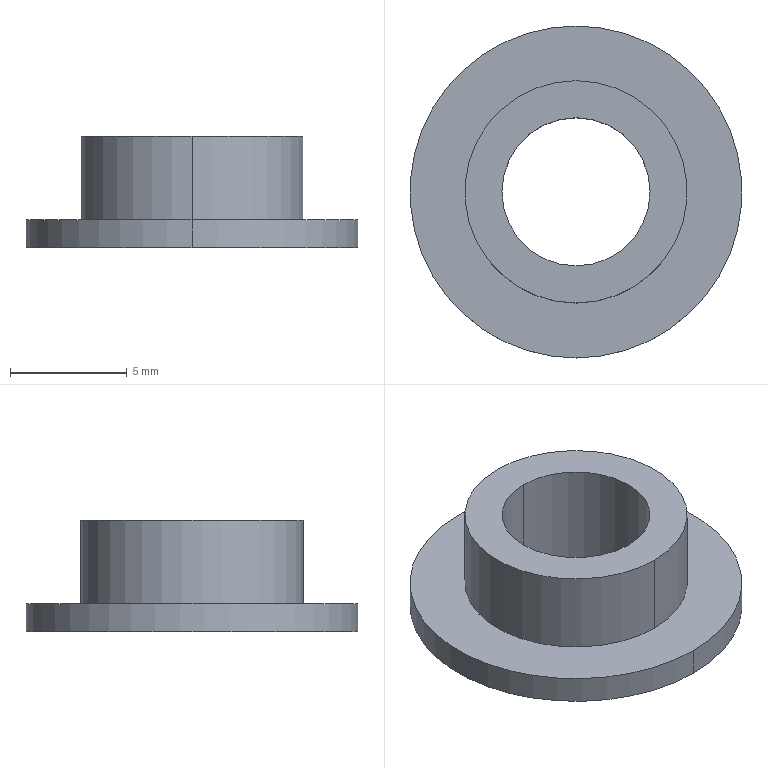Part | NX | features BREP 1 | 1 solid | 9 faces | box 14.224 x 14.224 x 4.763 mm | volume 293.165 mm3 | cylinder 6 | plane 3 | commonest cylinder face diameters 6.35 x2 9.525 x2 14.224 x2
STEP:
#1=CARTESIAN_POINT('',(0.,3.175,4.763));
#2=VERTEX_POINT('',#1);
#3=CARTESIAN_POINT('',(0.,-3.175,4.763));
#4=VERTEX_POINT('',#3);
#5=CARTESIAN_POINT('',(0.,0.,4.763));
#6=DIRECTION('',(0.,0.,1.));
#7=DIRECTION('',(0.,1.,0.));
#8=AXIS2_PLACEMENT_3D('',#5,#6,#7);
#9=CIRCLE('',#8,3.175);
#10=EDGE_CURVE('',#2,#4,#9,.T.);
#11=ORIENTED_EDGE('',*,*,#10,.T.);
#12=CARTESIAN_POINT('',(0.,-3.175,0.));
#13=VERTEX_POINT('',#12);
#14=CARTESIAN_POINT('',(0.,-3.175,0.));
#15=DIRECTION('',(0.,0.,1.));
#16=VECTOR('',#15,1000.);
#17=LINE('',#14,#16);
#18=EDGE_CURVE('',#4,#13,#17,.F.);
#19=ORIENTED_EDGE('',*,*,#18,.T.);
#20=CARTESIAN_POINT('',(0.,3.175,0.));
#21=VERTEX_POINT('',#20);
#22=CARTESIAN_POINT('',(0.,0.,0.));
#23=DIRECTION('',(0.,0.,1.));
#24=DIRECTION('',(0.,1.,0.));
#25=AXIS2_PLACEMENT_3D('',#22,#23,#24);
#26=CIRCLE('',#25,3.175);
#27=EDGE_CURVE('',#21,#13,#26,.T.);
#28=ORIENTED_EDGE('',*,*,#27,.F.);
#29=CARTESIAN_POINT('',(0.,3.175,0.));
#30=DIRECTION('',(0.,0.,1.));
#31=VECTOR('',#30,1000.);
#32=LINE('',#29,#31);
#33=EDGE_CURVE('',#2,#21,#32,.F.);
#34=ORIENTED_EDGE('',*,*,#33,.F.);
#35=EDGE_LOOP('',(#11,#19,#28,#34));
#36=FACE_BOUND('',#35,.T.);
#37=CARTESIAN_POINT('',(0.,0.,-0.2381));
#38=DIRECTION('',(0.,0.,1.));
#39=DIRECTION('',(0.,-1.,0.));
#40=AXIS2_PLACEMENT_3D('',#37,#38,#39);
#41=CYLINDRICAL_SURFACE('',#40,3.175);
#42=ADVANCED_FACE('',(#36),#41,.F.);
#43=CARTESIAN_POINT('',(0.,0.,0.));
#44=DIRECTION('',(0.,0.,-1.));
#45=DIRECTION('',(0.,1.,0.));
#46=AXIS2_PLACEMENT_3D('',#43,#44,#45);
#47=CIRCLE('',#46,3.175);
#48=EDGE_CURVE('',#21,#13,#47,.T.);
#49=ORIENTED_EDGE('',*,*,#48,.T.);
#50=ORIENTED_EDGE('',*,*,#18,.F.);
#51=CARTESIAN_POINT('',(0.,0.,4.763));
#52=DIRECTION('',(0.,0.,-1.));
#53=DIRECTION('',(0.,1.,0.));
#54=AXIS2_PLACEMENT_3D('',#51,#52,#53);
#55=CIRCLE('',#54,3.175);
#56=EDGE_CURVE('',#2,#4,#55,.T.);
#57=ORIENTED_EDGE('',*,*,#56,.F.);
#58=ORIENTED_EDGE('',*,*,#33,.T.);
#59=EDGE_LOOP('',(#49,#50,#57,#58));
#60=FACE_BOUND('',#59,.T.);
#61=CARTESIAN_POINT('',(0.,0.,-0.2381));
#62=DIRECTION('',(0.,0.,1.));
#63=DIRECTION('',(0.,-1.,0.));
#64=AXIS2_PLACEMENT_3D('',#61,#62,#63);
#65=CYLINDRICAL_SURFACE('',#64,3.175);
#66=ADVANCED_FACE('',(#60),#65,.F.);
#67=CARTESIAN_POINT('',(0.,4.763,4.763));
#68=VERTEX_POINT('',#67);
#69=CARTESIAN_POINT('',(0.,-4.763,4.763));
#70=VERTEX_POINT('',#69);
#71=CARTESIAN_POINT('',(0.,0.,4.763));
#72=DIRECTION('',(0.,0.,-1.));
#73=DIRECTION('',(0.,1.,0.));
#74=AXIS2_PLACEMENT_3D('',#71,#72,#73);
#75=CIRCLE('',#74,4.763);
#76=EDGE_CURVE('',#68,#70,#75,.T.);
#77=ORIENTED_EDGE('',*,*,#76,.F.);
#78=CARTESIAN_POINT('',(0.,0.,4.763));
#79=DIRECTION('',(0.,0.,1.));
#80=DIRECTION('',(0.,1.,0.));
#81=AXIS2_PLACEMENT_3D('',#78,#79,#80);
#82=CIRCLE('',#81,4.763);
#83=EDGE_CURVE('',#68,#70,#82,.T.);
#84=ORIENTED_EDGE('',*,*,#83,.T.);
#85=EDGE_LOOP('',(#77,#84));
#86=FACE_BOUND('',#85,.T.);
#87=ORIENTED_EDGE('',*,*,#10,.F.);
#88=ORIENTED_EDGE('',*,*,#56,.T.);
#89=EDGE_LOOP('',(#87,#88));
#90=FACE_BOUND('',#89,.T.);
#91=CARTESIAN_POINT('',(0.,0.,4.763));
#92=DIRECTION('',(0.,0.,1.));
#93=DIRECTION('',(1.,0.,0.));
#94=AXIS2_PLACEMENT_3D('',#91,#92,#93);
#95=PLANE('',#94);
#96=ADVANCED_FACE('',(#86,#90),#95,.T.);
#97=CARTESIAN_POINT('',(0.,4.763,1.194));
#98=VERTEX_POINT('',#97);
#99=CARTESIAN_POINT('',(0.,-4.763,1.194));
#100=VERTEX_POINT('',#99);
#101=CARTESIAN_POINT('',(0.,0.,1.194));
#102=DIRECTION('',(0.,0.,1.));
#103=DIRECTION('',(0.,1.,0.));
#104=AXIS2_PLACEMENT_3D('',#101,#102,#103);
#105=CIRCLE('',#104,4.763);
#106=EDGE_CURVE('',#98,#100,#105,.T.);
#107=ORIENTED_EDGE('',*,*,#106,.T.);
#108=CARTESIAN_POINT('',(0.,-4.763,4.763));
#109=DIRECTION('',(0.,0.,-1.));
#110=VECTOR('',#109,1000.);
#111=LINE('',#108,#110);
#112=EDGE_CURVE('',#100,#70,#111,.F.);
#113=ORIENTED_EDGE('',*,*,#112,.T.);
#114=ORIENTED_EDGE('',*,*,#83,.F.);
#115=CARTESIAN_POINT('',(0.,4.763,4.763));
#116=DIRECTION('',(0.,0.,-1.));
#117=VECTOR('',#116,1000.);
#118=LINE('',#115,#117);
#119=EDGE_CURVE('',#98,#68,#118,.F.);
#120=ORIENTED_EDGE('',*,*,#119,.F.);
#121=EDGE_LOOP('',(#107,#113,#114,#120));
#122=FACE_BOUND('',#121,.T.);
#123=CARTESIAN_POINT('',(0.,0.,-0.2381));
#124=DIRECTION('',(0.,0.,1.));
#125=DIRECTION('',(0.,-1.,0.));
#126=AXIS2_PLACEMENT_3D('',#123,#124,#125);
#127=CYLINDRICAL_SURFACE('',#126,4.763);
#128=ADVANCED_FACE('',(#122),#127,.T.);
#129=ORIENTED_EDGE('',*,*,#76,.T.);
#130=ORIENTED_EDGE('',*,*,#112,.F.);
#131=CARTESIAN_POINT('',(0.,0.,1.194));
#132=DIRECTION('',(0.,0.,-1.));
#133=DIRECTION('',(0.,1.,0.));
#134=AXIS2_PLACEMENT_3D('',#131,#132,#133);
#135=CIRCLE('',#134,4.763);
#136=EDGE_CURVE('',#98,#100,#135,.T.);
#137=ORIENTED_EDGE('',*,*,#136,.F.);
#138=ORIENTED_EDGE('',*,*,#119,.T.);
#139=EDGE_LOOP('',(#129,#130,#137,#138));
#140=FACE_BOUND('',#139,.T.);
#141=CARTESIAN_POINT('',(0.,0.,-0.2381));
#142=DIRECTION('',(0.,0.,1.));
#143=DIRECTION('',(0.,-1.,0.));
#144=AXIS2_PLACEMENT_3D('',#141,#142,#143);
#145=CYLINDRICAL_SURFACE('',#144,4.763);
#146=ADVANCED_FACE('',(#140),#145,.T.);
#147=CARTESIAN_POINT('',(0.,7.112,1.194));
#148=VERTEX_POINT('',#147);
#149=CARTESIAN_POINT('',(0.,-7.112,1.194));
#150=VERTEX_POINT('',#149);
#151=CARTESIAN_POINT('',(0.,0.,1.194));
#152=DIRECTION('',(0.,0.,-1.));
#153=DIRECTION('',(0.,1.,0.));
#154=AXIS2_PLACEMENT_3D('',#151,#152,#153);
#155=CIRCLE('',#154,7.112);
#156=EDGE_CURVE('',#148,#150,#155,.T.);
#157=ORIENTED_EDGE('',*,*,#156,.F.);
#158=CARTESIAN_POINT('',(0.,0.,1.194));
#159=DIRECTION('',(0.,0.,1.));
#160=DIRECTION('',(0.,1.,0.));
#161=AXIS2_PLACEMENT_3D('',#158,#159,#160);
#162=CIRCLE('',#161,7.112);
#163=EDGE_CURVE('',#148,#150,#162,.T.);
#164=ORIENTED_EDGE('',*,*,#163,.T.);
#165=EDGE_LOOP('',(#157,#164));
#166=FACE_BOUND('',#165,.T.);
#167=ORIENTED_EDGE('',*,*,#106,.F.);
#168=ORIENTED_EDGE('',*,*,#136,.T.);
#169=EDGE_LOOP('',(#167,#168));
#170=FACE_BOUND('',#169,.T.);
#171=CARTESIAN_POINT('',(0.,0.,1.194));
#172=DIRECTION('',(0.,0.,1.));
#173=DIRECTION('',(1.,0.,0.));
#174=AXIS2_PLACEMENT_3D('',#171,#172,#173);
#175=PLANE('',#174);
#176=ADVANCED_FACE('',(#166,#170),#175,.T.);
#177=CARTESIAN_POINT('',(0.,7.112,0.));
#178=VERTEX_POINT('',#177);
#179=CARTESIAN_POINT('',(0.,-7.112,0.));
#180=VERTEX_POINT('',#179);
#181=CARTESIAN_POINT('',(0.,0.,0.));
#182=DIRECTION('',(0.,0.,1.));
#183=DIRECTION('',(0.,1.,0.));
#184=AXIS2_PLACEMENT_3D('',#181,#182,#183);
#185=CIRCLE('',#184,7.112);
#186=EDGE_CURVE('',#178,#180,#185,.T.);
#187=ORIENTED_EDGE('',*,*,#186,.T.);
#188=CARTESIAN_POINT('',(0.,-7.112,1.194));
#189=DIRECTION('',(0.,0.,-1.));
#190=VECTOR('',#189,1000.);
#191=LINE('',#188,#190);
#192=EDGE_CURVE('',#180,#150,#191,.F.);
#193=ORIENTED_EDGE('',*,*,#192,.T.);
#194=ORIENTED_EDGE('',*,*,#163,.F.);
#195=CARTESIAN_POINT('',(0.,7.112,1.194));
#196=DIRECTION('',(0.,0.,-1.));
#197=VECTOR('',#196,1000.);
#198=LINE('',#195,#197);
#199=EDGE_CURVE('',#178,#148,#198,.F.);
#200=ORIENTED_EDGE('',*,*,#199,.F.);
#201=EDGE_LOOP('',(#187,#193,#194,#200));
#202=FACE_BOUND('',#201,.T.);
#203=CARTESIAN_POINT('',(0.,0.,-0.2381));
#204=DIRECTION('',(0.,0.,1.));
#205=DIRECTION('',(0.,-1.,0.));
#206=AXIS2_PLACEMENT_3D('',#203,#204,#205);
#207=CYLINDRICAL_SURFACE('',#206,7.112);
#208=ADVANCED_FACE('',(#202),#207,.T.);
#209=ORIENTED_EDGE('',*,*,#156,.T.);
#210=ORIENTED_EDGE('',*,*,#192,.F.);
#211=CARTESIAN_POINT('',(0.,0.,0.));
#212=DIRECTION('',(0.,0.,-1.));
#213=DIRECTION('',(0.,1.,0.));
#214=AXIS2_PLACEMENT_3D('',#211,#212,#213);
#215=CIRCLE('',#214,7.112);
#216=EDGE_CURVE('',#178,#180,#215,.T.);
#217=ORIENTED_EDGE('',*,*,#216,.F.);
#218=ORIENTED_EDGE('',*,*,#199,.T.);
#219=EDGE_LOOP('',(#209,#210,#217,#218));
#220=FACE_BOUND('',#219,.T.);
#221=CARTESIAN_POINT('',(0.,0.,-0.2381));
#222=DIRECTION('',(0.,0.,1.));
#223=DIRECTION('',(0.,-1.,0.));
#224=AXIS2_PLACEMENT_3D('',#221,#222,#223);
#225=CYLINDRICAL_SURFACE('',#224,7.112);
#226=ADVANCED_FACE('',(#220),#225,.T.);
#227=ORIENTED_EDGE('',*,*,#186,.F.);
#228=ORIENTED_EDGE('',*,*,#216,.T.);
#229=EDGE_LOOP('',(#227,#228));
#230=FACE_BOUND('',#229,.T.);
#231=ORIENTED_EDGE('',*,*,#48,.F.);
#232=ORIENTED_EDGE('',*,*,#27,.T.);
#233=EDGE_LOOP('',(#231,#232));
#234=FACE_BOUND('',#233,.T.);
#235=CARTESIAN_POINT('',(0.,0.,0.));
#236=DIRECTION('',(0.,0.,1.));
#237=DIRECTION('',(1.,0.,0.));
#238=AXIS2_PLACEMENT_3D('',#235,#236,#237);
#239=PLANE('',#238);
#240=ADVANCED_FACE('',(#230,#234),#239,.F.);
#241=CLOSED_SHELL('',(#42,#66,#96,#128,#146,#176,#208,#226,#240));
#242=MANIFOLD_SOLID_BREP('',#241);
#243=(LENGTH_UNIT()NAMED_UNIT(*)SI_UNIT(.MILLI.,.METRE.));
#244=UNCERTAINTY_MEASURE_WITH_UNIT(LENGTH_MEASURE(0.00001),#243,'','');
#245=(NAMED_UNIT(*)PLANE_ANGLE_UNIT()SI_UNIT($,.RADIAN.));
#246=(NAMED_UNIT(*)SI_UNIT($,.STERADIAN.)SOLID_ANGLE_UNIT());
#247=(GEOMETRIC_REPRESENTATION_CONTEXT(3)GLOBAL_UNCERTAINTY_ASSIGNED_CONTEXT((#244))GLOBAL_UNIT_ASSIGNED_CONTEXT((#243,#245,#246))REPRESENTATION_CONTEXT('',''));
#248=ADVANCED_BREP_SHAPE_REPRESENTATION('',(#242),#247);